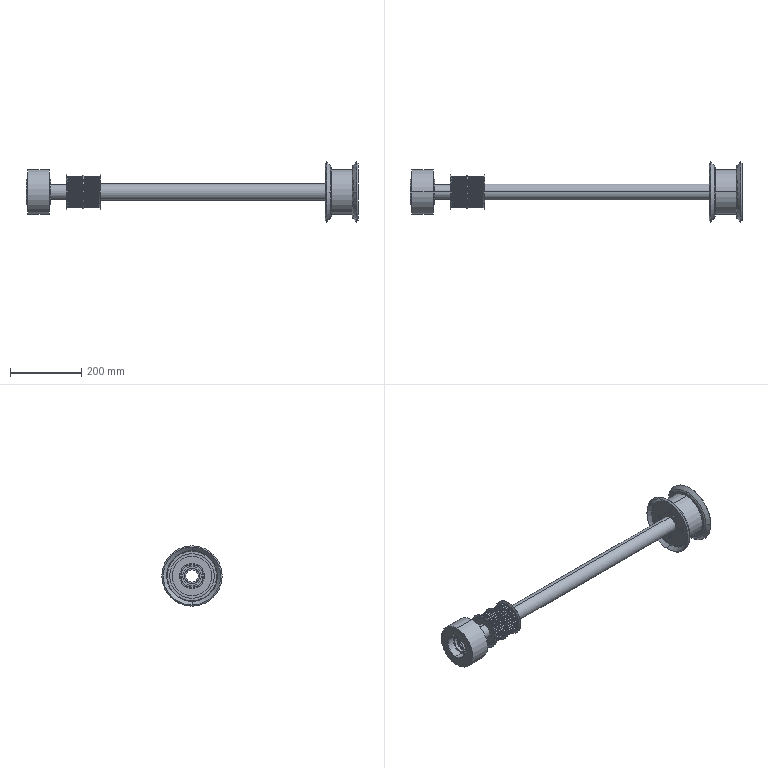Part | SolidWorks | 15 solids | 1500 faces | box 930.556 x 169.042 x 169.042 mm | volume 2373220 mm3 | cylinder 738 | plane 422 | cone 216 | spline 124 | commonest cylinder face diameters 6 x200 1.6 x168 5.14 x168 85.208 x70 5 x16 6.6 x16